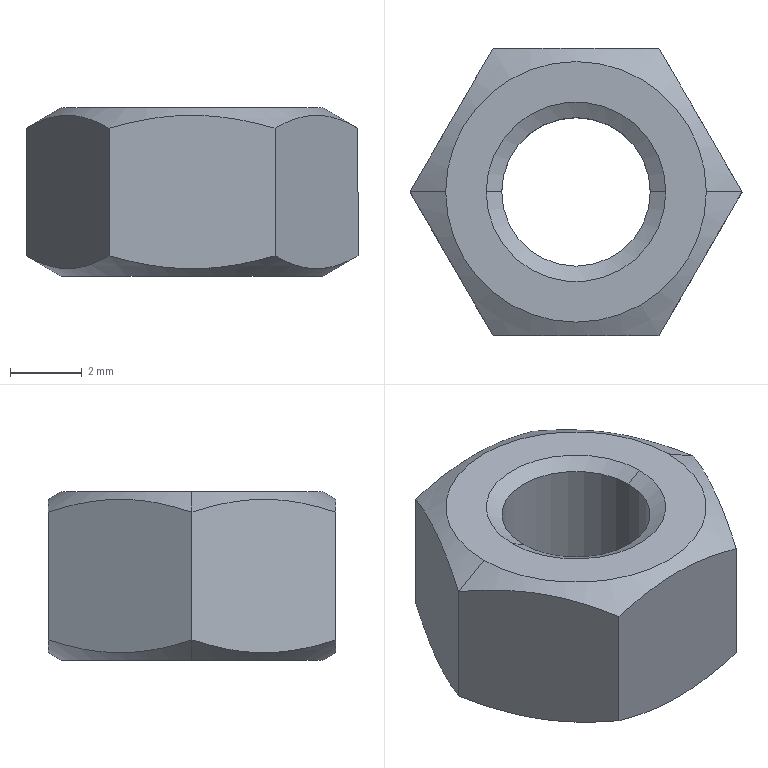Part | SolidWorks | features RevCut 2, Chamfer 1, Extrusion 1, LPattern 1 | 1 solid | 18 faces | box 9.238 x 8 x 4.7 mm | volume 190.603 mm3 | cone 8 | plane 8 | cylinder 2 | commonest cylinder face diameters 4.134 x2
STEP:
#1=CARTESIAN_POINT('',(-2.067,0.,-0.25));
#2=VERTEX_POINT('',#1);
#3=CARTESIAN_POINT('',(2.067,0.,-0.25));
#4=VERTEX_POINT('',#3);
#5=CARTESIAN_POINT('',(0.,0.,-0.25));
#6=DIRECTION('',(0.,0.,1.));
#7=DIRECTION('',(-1.,0.,0.));
#8=AXIS2_PLACEMENT_3D('',#5,#6,#7);
#9=CIRCLE('',#8,2.067);
#10=EDGE_CURVE('',#2,#4,#9,.T.);
#11=ORIENTED_EDGE('',*,*,#10,.F.);
#12=CARTESIAN_POINT('',(-2.5,0.,0.));
#13=VERTEX_POINT('',#12);
#14=CARTESIAN_POINT('',(-2.067,0.,-0.25));
#15=DIRECTION('',(-0.866,0.,0.5));
#16=VECTOR('',#15,1000.);
#17=LINE('',#14,#16);
#18=EDGE_CURVE('',#2,#13,#17,.T.);
#19=ORIENTED_EDGE('',*,*,#18,.T.);
#20=CARTESIAN_POINT('',(2.5,0.,0.));
#21=VERTEX_POINT('',#20);
#22=CARTESIAN_POINT('',(0.,0.,0.));
#23=DIRECTION('',(0.,0.,-1.));
#24=DIRECTION('',(-1.,0.,0.));
#25=AXIS2_PLACEMENT_3D('',#22,#23,#24);
#26=CIRCLE('',#25,2.5);
#27=EDGE_CURVE('',#21,#13,#26,.T.);
#28=ORIENTED_EDGE('',*,*,#27,.F.);
#29=CARTESIAN_POINT('',(2.067,0.,-0.25));
#30=DIRECTION('',(0.866,0.,0.5));
#31=VECTOR('',#30,1000.);
#32=LINE('',#29,#31);
#33=EDGE_CURVE('',#4,#21,#32,.T.);
#34=ORIENTED_EDGE('',*,*,#33,.F.);
#35=EDGE_LOOP('',(#11,#19,#28,#34));
#36=FACE_OUTER_BOUND('',#35,.T.);
#37=CARTESIAN_POINT('',(0.,0.,-0.25));
#38=DIRECTION('',(0.,0.,1.));
#39=DIRECTION('',(1.,0.,0.));
#40=AXIS2_PLACEMENT_3D('',#37,#38,#39);
#41=CONICAL_SURFACE('',#40,2.067,1.047);
#42=ADVANCED_FACE('',(#36),#41,.F.);
#43=CARTESIAN_POINT('',(2.067,0.,-4.267));
#44=VERTEX_POINT('',#43);
#45=CARTESIAN_POINT('',(-2.067,0.,-4.267));
#46=VERTEX_POINT('',#45);
#47=CARTESIAN_POINT('',(0.,0.,-4.267));
#48=DIRECTION('',(0.,0.,-1.));
#49=DIRECTION('',(-1.,0.,0.));
#50=AXIS2_PLACEMENT_3D('',#47,#48,#49);
#51=CIRCLE('',#50,2.067);
#52=EDGE_CURVE('',#44,#46,#51,.T.);
#53=ORIENTED_EDGE('',*,*,#52,.F.);
#54=CARTESIAN_POINT('',(2.317,0.,-4.7));
#55=VERTEX_POINT('',#54);
#56=CARTESIAN_POINT('',(2.317,0.,-4.7));
#57=DIRECTION('',(0.5,0.,-0.866));
#58=VECTOR('',#57,1000.);
#59=LINE('',#56,#58);
#60=EDGE_CURVE('',#44,#55,#59,.T.);
#61=ORIENTED_EDGE('',*,*,#60,.T.);
#62=CARTESIAN_POINT('',(-2.317,0.,-4.7));
#63=VERTEX_POINT('',#62);
#64=CARTESIAN_POINT('',(0.,0.,-4.7));
#65=DIRECTION('',(0.,0.,1.));
#66=DIRECTION('',(-1.,0.,0.));
#67=AXIS2_PLACEMENT_3D('',#64,#65,#66);
#68=CIRCLE('',#67,2.317);
#69=EDGE_CURVE('',#63,#55,#68,.T.);
#70=ORIENTED_EDGE('',*,*,#69,.F.);
#71=CARTESIAN_POINT('',(-2.317,0.,-4.7));
#72=DIRECTION('',(-0.5,0.,-0.866));
#73=VECTOR('',#72,1000.);
#74=LINE('',#71,#73);
#75=EDGE_CURVE('',#46,#63,#74,.T.);
#76=ORIENTED_EDGE('',*,*,#75,.F.);
#77=EDGE_LOOP('',(#53,#61,#70,#76));
#78=FACE_OUTER_BOUND('',#77,.T.);
#79=CARTESIAN_POINT('',(0.,0.,-4.7));
#80=DIRECTION('',(0.,0.,-1.));
#81=DIRECTION('',(-1.,0.,0.));
#82=AXIS2_PLACEMENT_3D('',#79,#80,#81);
#83=CONICAL_SURFACE('',#82,2.317,0.5236);
#84=ADVANCED_FACE('',(#78),#83,.F.);
#85=CARTESIAN_POINT('',(-3.625,0.,0.));
#86=VERTEX_POINT('',#85);
#87=CARTESIAN_POINT('',(3.625,0.,0.));
#88=VERTEX_POINT('',#87);
#89=CARTESIAN_POINT('',(0.,0.,0.));
#90=DIRECTION('',(0.,0.,-1.));
#91=DIRECTION('',(-1.,0.,0.));
#92=AXIS2_PLACEMENT_3D('',#89,#90,#91);
#93=CIRCLE('',#92,3.625);
#94=EDGE_CURVE('',#86,#88,#93,.T.);
#95=ORIENTED_EDGE('',*,*,#94,.T.);
#96=CARTESIAN_POINT('',(4.619,0.,-0.5738));
#97=VERTEX_POINT('',#96);
#98=CARTESIAN_POINT('',(3.625,0.,0.));
#99=DIRECTION('',(0.866,0.,-0.5));
#100=VECTOR('',#99,1000.);
#101=LINE('',#98,#100);
#102=EDGE_CURVE('',#88,#97,#101,.T.);
#103=ORIENTED_EDGE('',*,*,#102,.T.);
#104=CARTESIAN_POINT('',(2.309,4.,-0.5738));
#105=VERTEX_POINT('',#104);
#106=CARTESIAN_POINT('',(4.619,0.,-0.5738));
#107=CARTESIAN_POINT('',(4.242,0.6531,-0.3561));
#108=CARTESIAN_POINT('',(3.859,1.316,-0.217));
#109=CARTESIAN_POINT('',(3.27,2.336,-0.2163));
#110=CARTESIAN_POINT('',(3.074,2.676,-0.2504));
#111=CARTESIAN_POINT('',(2.689,3.343,-0.3748));
#112=CARTESIAN_POINT('',(2.498,3.673,-0.4648));
#113=CARTESIAN_POINT('',(2.309,4.,-0.5738));
#114=B_SPLINE_CURVE_WITH_KNOTS('',3,(#106,#107,#108,#109,#110,#111,#112,#113),.UNSPECIFIED.,.F.,.F.,(4,2,2,4),(0.000000238,0.002333,0.003499,0.004665),.UNSPECIFIED.);
#115=EDGE_CURVE('',#97,#105,#114,.T.);
#116=ORIENTED_EDGE('',*,*,#115,.T.);
#117=CARTESIAN_POINT('',(-2.309,4.,-0.5738));
#118=VERTEX_POINT('',#117);
#119=CARTESIAN_POINT('',(2.309,4.,-0.5738));
#120=CARTESIAN_POINT('',(1.936,4.,-0.466));
#121=CARTESIAN_POINT('',(1.558,4.,-0.3762));
#122=CARTESIAN_POINT('',(0.7865,4.,-0.251));
#123=CARTESIAN_POINT('',(0.3909,4.,-0.2165));
#124=CARTESIAN_POINT('',(-0.3896,4.,-0.2165));
#125=CARTESIAN_POINT('',(-0.7775,4.,-0.25));
#126=CARTESIAN_POINT('',(-1.549,4.,-0.3744));
#127=CARTESIAN_POINT('',(-1.934,4.,-0.4653));
#128=CARTESIAN_POINT('',(-2.309,4.,-0.5738));
#129=B_SPLINE_CURVE_WITH_KNOTS('',3,(#119,#120,#121,#122,#123,#124,#125,#126,#127,#128),.UNSPECIFIED.,.F.,.F.,(4,2,2,2,4),(0.001729,0.002894,0.00406,0.005225,0.006391),.UNSPECIFIED.);
#130=EDGE_CURVE('',#105,#118,#129,.T.);
#131=ORIENTED_EDGE('',*,*,#130,.T.);
#132=CARTESIAN_POINT('',(-4.619,0.,-0.5738));
#133=VERTEX_POINT('',#132);
#134=CARTESIAN_POINT('',(-2.309,4.,-0.5738));
#135=CARTESIAN_POINT('',(-2.686,3.347,-0.3561));
#136=CARTESIAN_POINT('',(-3.069,2.684,-0.217));
#137=CARTESIAN_POINT('',(-3.658,1.664,-0.2163));
#138=CARTESIAN_POINT('',(-3.854,1.324,-0.2504));
#139=CARTESIAN_POINT('',(-4.24,0.6567,-0.3748));
#140=CARTESIAN_POINT('',(-4.43,0.327,-0.4648));
#141=CARTESIAN_POINT('',(-4.619,0.,-0.5738));
#142=B_SPLINE_CURVE_WITH_KNOTS('',3,(#134,#135,#136,#137,#138,#139,#140,#141),.UNSPECIFIED.,.F.,.F.,(4,2,2,4),(0.000000238,0.002333,0.003499,0.004665),.UNSPECIFIED.);
#143=EDGE_CURVE('',#118,#133,#142,.T.);
#144=ORIENTED_EDGE('',*,*,#143,.T.);
#145=CARTESIAN_POINT('',(-3.625,0.,0.));
#146=DIRECTION('',(-0.866,0.,-0.5));
#147=VECTOR('',#146,1000.);
#148=LINE('',#145,#147);
#149=EDGE_CURVE('',#86,#133,#148,.T.);
#150=ORIENTED_EDGE('',*,*,#149,.F.);
#151=EDGE_LOOP('',(#95,#103,#116,#131,#144,#150));
#152=FACE_OUTER_BOUND('',#151,.T.);
#153=CARTESIAN_POINT('',(0.,0.,0.));
#154=DIRECTION('',(0.,0.,-1.));
#155=DIRECTION('',(-1.,0.,0.));
#156=AXIS2_PLACEMENT_3D('',#153,#154,#155);
#157=CONICAL_SURFACE('',#156,3.625,1.047);
#158=ADVANCED_FACE('',(#152),#157,.T.);
#159=CARTESIAN_POINT('',(-3.625,0.,-4.7));
#160=VERTEX_POINT('',#159);
#161=CARTESIAN_POINT('',(3.625,0.,-4.7));
#162=VERTEX_POINT('',#161);
#163=CARTESIAN_POINT('',(0.,0.,-4.7));
#164=DIRECTION('',(0.,0.,-1.));
#165=DIRECTION('',(-1.,0.,0.));
#166=AXIS2_PLACEMENT_3D('',#163,#164,#165);
#167=CIRCLE('',#166,3.625);
#168=EDGE_CURVE('',#160,#162,#167,.T.);
#169=ORIENTED_EDGE('',*,*,#168,.F.);
#170=CARTESIAN_POINT('',(-4.619,0.,-4.126));
#171=VERTEX_POINT('',#170);
#172=CARTESIAN_POINT('',(-4.619,0.,-4.126));
#173=DIRECTION('',(-0.866,0.,0.5));
#174=VECTOR('',#173,1000.);
#175=LINE('',#172,#174);
#176=EDGE_CURVE('',#160,#171,#175,.T.);
#177=ORIENTED_EDGE('',*,*,#176,.T.);
#178=CARTESIAN_POINT('',(-2.309,4.,-4.126));
#179=VERTEX_POINT('',#178);
#180=CARTESIAN_POINT('',(-4.619,0.,-4.126));
#181=CARTESIAN_POINT('',(-4.242,0.6531,-4.344));
#182=CARTESIAN_POINT('',(-3.859,1.316,-4.483));
#183=CARTESIAN_POINT('',(-3.27,2.336,-4.484));
#184=CARTESIAN_POINT('',(-3.074,2.676,-4.45));
#185=CARTESIAN_POINT('',(-2.689,3.343,-4.325));
#186=CARTESIAN_POINT('',(-2.498,3.673,-4.235));
#187=CARTESIAN_POINT('',(-2.309,4.,-4.126));
#188=B_SPLINE_CURVE_WITH_KNOTS('',3,(#180,#181,#182,#183,#184,#185,#186,#187),.UNSPECIFIED.,.F.,.F.,(4,2,2,4),(0.000000238,0.002333,0.003499,0.004665),.UNSPECIFIED.);
#189=EDGE_CURVE('',#171,#179,#188,.T.);
#190=ORIENTED_EDGE('',*,*,#189,.T.);
#191=CARTESIAN_POINT('',(2.309,4.,-4.126));
#192=VERTEX_POINT('',#191);
#193=CARTESIAN_POINT('',(-2.309,4.,-4.126));
#194=CARTESIAN_POINT('',(-1.934,4.,-4.235));
#195=CARTESIAN_POINT('',(-1.549,4.,-4.326));
#196=CARTESIAN_POINT('',(-0.7775,4.,-4.45));
#197=CARTESIAN_POINT('',(-0.3896,4.,-4.484));
#198=CARTESIAN_POINT('',(0.3909,4.,-4.483));
#199=CARTESIAN_POINT('',(0.7865,4.,-4.449));
#200=CARTESIAN_POINT('',(1.558,4.,-4.324));
#201=CARTESIAN_POINT('',(1.936,4.,-4.234));
#202=CARTESIAN_POINT('',(2.309,4.,-4.126));
#203=B_SPLINE_CURVE_WITH_KNOTS('',3,(#193,#194,#195,#196,#197,#198,#199,#200,#201,#202),.UNSPECIFIED.,.F.,.F.,(4,2,2,2,4),(0.004087,0.005255,0.006424,0.007592,0.00876),.UNSPECIFIED.);
#204=EDGE_CURVE('',#179,#192,#203,.T.);
#205=ORIENTED_EDGE('',*,*,#204,.T.);
#206=CARTESIAN_POINT('',(4.619,0.,-4.126));
#207=VERTEX_POINT('',#206);
#208=CARTESIAN_POINT('',(2.309,4.,-4.126));
#209=CARTESIAN_POINT('',(2.686,3.347,-4.344));
#210=CARTESIAN_POINT('',(3.069,2.684,-4.483));
#211=CARTESIAN_POINT('',(3.658,1.664,-4.484));
#212=CARTESIAN_POINT('',(3.854,1.324,-4.45));
#213=CARTESIAN_POINT('',(4.24,0.6567,-4.325));
#214=CARTESIAN_POINT('',(4.43,0.327,-4.235));
#215=CARTESIAN_POINT('',(4.619,0.,-4.126));
#216=B_SPLINE_CURVE_WITH_KNOTS('',3,(#208,#209,#210,#211,#212,#213,#214,#215),.UNSPECIFIED.,.F.,.F.,(4,2,2,4),(0.000000238,0.002333,0.003499,0.004665),.UNSPECIFIED.);
#217=EDGE_CURVE('',#192,#207,#216,.T.);
#218=ORIENTED_EDGE('',*,*,#217,.T.);
#219=CARTESIAN_POINT('',(4.619,0.,-4.126));
#220=DIRECTION('',(0.866,0.,0.5));
#221=VECTOR('',#220,1000.);
#222=LINE('',#219,#221);
#223=EDGE_CURVE('',#162,#207,#222,.T.);
#224=ORIENTED_EDGE('',*,*,#223,.F.);
#225=EDGE_LOOP('',(#169,#177,#190,#205,#218,#224));
#226=FACE_OUTER_BOUND('',#225,.T.);
#227=CARTESIAN_POINT('',(0.,0.,-4.126));
#228=DIRECTION('',(0.,0.,1.));
#229=DIRECTION('',(1.,0.,0.));
#230=AXIS2_PLACEMENT_3D('',#227,#228,#229);
#231=CONICAL_SURFACE('',#230,4.619,1.047);
#232=ADVANCED_FACE('',(#226),#231,.T.);
#233=ORIENTED_EDGE('',*,*,#52,.T.);
#234=CARTESIAN_POINT('',(-2.067,0.,-4.7));
#235=DIRECTION('',(0.,0.,1.));
#236=VECTOR('',#235,1000.);
#237=LINE('',#234,#236);
#238=EDGE_CURVE('',#46,#2,#237,.T.);
#239=ORIENTED_EDGE('',*,*,#238,.T.);
#240=ORIENTED_EDGE('',*,*,#10,.T.);
#241=CARTESIAN_POINT('',(2.067,0.,-4.7));
#242=DIRECTION('',(0.,0.,1.));
#243=VECTOR('',#242,1000.);
#244=LINE('',#241,#243);
#245=EDGE_CURVE('',#44,#4,#244,.T.);
#246=ORIENTED_EDGE('',*,*,#245,.F.);
#247=EDGE_LOOP('',(#233,#239,#240,#246));
#248=FACE_OUTER_BOUND('',#247,.T.);
#249=CARTESIAN_POINT('',(0.,0.,-4.7));
#250=DIRECTION('',(0.,0.,1.));
#251=DIRECTION('',(1.,0.,0.));
#252=AXIS2_PLACEMENT_3D('',#249,#250,#251);
#253=CYLINDRICAL_SURFACE('',#252,2.067);
#254=ADVANCED_FACE('',(#248),#253,.F.);
#255=CARTESIAN_POINT('',(2.309,-4.,-0.5738));
#256=VERTEX_POINT('',#255);
#257=CARTESIAN_POINT('',(2.309,-4.,-0.5738));
#258=CARTESIAN_POINT('',(2.686,-3.347,-0.3561));
#259=CARTESIAN_POINT('',(3.069,-2.684,-0.217));
#260=CARTESIAN_POINT('',(3.658,-1.664,-0.2163));
#261=CARTESIAN_POINT('',(3.854,-1.324,-0.2504));
#262=CARTESIAN_POINT('',(4.24,-0.6567,-0.3748));
#263=CARTESIAN_POINT('',(4.43,-0.327,-0.4648));
#264=CARTESIAN_POINT('',(4.619,0.,-0.5738));
#265=B_SPLINE_CURVE_WITH_KNOTS('',3,(#257,#258,#259,#260,#261,#262,#263,#264),.UNSPECIFIED.,.F.,.F.,(4,2,2,4),(0.000000238,0.002333,0.003499,0.004665),.UNSPECIFIED.);
#266=EDGE_CURVE('',#256,#97,#265,.T.);
#267=ORIENTED_EDGE('',*,*,#266,.F.);
#268=CARTESIAN_POINT('',(2.309,-4.,-4.126));
#269=VERTEX_POINT('',#268);
#270=CARTESIAN_POINT('',(2.309,-4.,-4.7));
#271=DIRECTION('',(0.,0.,1.));
#272=VECTOR('',#271,1000.);
#273=LINE('',#270,#272);
#274=EDGE_CURVE('',#269,#256,#273,.T.);
#275=ORIENTED_EDGE('',*,*,#274,.F.);
#276=CARTESIAN_POINT('',(4.619,0.,-4.126));
#277=CARTESIAN_POINT('',(4.242,-0.6531,-4.344));
#278=CARTESIAN_POINT('',(3.859,-1.316,-4.483));
#279=CARTESIAN_POINT('',(3.27,-2.336,-4.484));
#280=CARTESIAN_POINT('',(3.074,-2.676,-4.45));
#281=CARTESIAN_POINT('',(2.689,-3.343,-4.325));
#282=CARTESIAN_POINT('',(2.498,-3.673,-4.235));
#283=CARTESIAN_POINT('',(2.309,-4.,-4.126));
#284=B_SPLINE_CURVE_WITH_KNOTS('',3,(#276,#277,#278,#279,#280,#281,#282,#283),.UNSPECIFIED.,.F.,.F.,(4,2,2,4),(0.000000238,0.002333,0.003499,0.004665),.UNSPECIFIED.);
#285=EDGE_CURVE('',#207,#269,#284,.T.);
#286=ORIENTED_EDGE('',*,*,#285,.F.);
#287=CARTESIAN_POINT('',(4.619,0.,-4.7));
#288=DIRECTION('',(0.,0.,1.));
#289=VECTOR('',#288,1000.);
#290=LINE('',#287,#289);
#291=EDGE_CURVE('',#207,#97,#290,.T.);
#292=ORIENTED_EDGE('',*,*,#291,.T.);
#293=EDGE_LOOP('',(#267,#275,#286,#292));
#294=FACE_OUTER_BOUND('',#293,.T.);
#295=CARTESIAN_POINT('',(2.309,-4.,-4.7));
#296=DIRECTION('',(0.866,-0.5,0.));
#297=DIRECTION('',(0.5,0.866,0.));
#298=AXIS2_PLACEMENT_3D('',#295,#296,#297);
#299=PLANE('',#298);
#300=ADVANCED_FACE('',(#294),#299,.T.);
#301=CARTESIAN_POINT('',(-2.309,-4.,-0.5738));
#302=VERTEX_POINT('',#301);
#303=CARTESIAN_POINT('',(-2.309,-4.,-0.5738));
#304=CARTESIAN_POINT('',(-1.934,-4.,-0.4653));
#305=CARTESIAN_POINT('',(-1.549,-4.,-0.3744));
#306=CARTESIAN_POINT('',(-0.7775,-4.,-0.25));
#307=CARTESIAN_POINT('',(-0.3896,-4.,-0.2165));
#308=CARTESIAN_POINT('',(0.3909,-4.,-0.2165));
#309=CARTESIAN_POINT('',(0.7865,-4.,-0.251));
#310=CARTESIAN_POINT('',(1.558,-4.,-0.3762));
#311=CARTESIAN_POINT('',(1.936,-4.,-0.466));
#312=CARTESIAN_POINT('',(2.309,-4.,-0.5738));
#313=B_SPLINE_CURVE_WITH_KNOTS('',3,(#303,#304,#305,#306,#307,#308,#309,#310,#311,#312),.UNSPECIFIED.,.F.,.F.,(4,2,2,2,4),(0.004087,0.005255,0.006424,0.007592,0.00876),.UNSPECIFIED.);
#314=EDGE_CURVE('',#302,#256,#313,.T.);
#315=ORIENTED_EDGE('',*,*,#314,.F.);
#316=CARTESIAN_POINT('',(-2.309,-4.,-4.126));
#317=VERTEX_POINT('',#316);
#318=CARTESIAN_POINT('',(-2.309,-4.,-4.7));
#319=DIRECTION('',(0.,0.,1.));
#320=VECTOR('',#319,1000.);
#321=LINE('',#318,#320);
#322=EDGE_CURVE('',#317,#302,#321,.T.);
#323=ORIENTED_EDGE('',*,*,#322,.F.);
#324=CARTESIAN_POINT('',(2.309,-4.,-4.126));
#325=CARTESIAN_POINT('',(1.936,-4.,-4.234));
#326=CARTESIAN_POINT('',(1.558,-4.,-4.324));
#327=CARTESIAN_POINT('',(0.7865,-4.,-4.449));
#328=CARTESIAN_POINT('',(0.3909,-4.,-4.483));
#329=CARTESIAN_POINT('',(-0.3896,-4.,-4.484));
#330=CARTESIAN_POINT('',(-0.7775,-4.,-4.45));
#331=CARTESIAN_POINT('',(-1.549,-4.,-4.326));
#332=CARTESIAN_POINT('',(-1.934,-4.,-4.235));
#333=CARTESIAN_POINT('',(-2.309,-4.,-4.126));
#334=B_SPLINE_CURVE_WITH_KNOTS('',3,(#324,#325,#326,#327,#328,#329,#330,#331,#332,#333),.UNSPECIFIED.,.F.,.F.,(4,2,2,2,4),(0.001729,0.002894,0.00406,0.005225,0.006391),.UNSPECIFIED.);
#335=EDGE_CURVE('',#269,#317,#334,.T.);
#336=ORIENTED_EDGE('',*,*,#335,.F.);
#337=ORIENTED_EDGE('',*,*,#274,.T.);
#338=EDGE_LOOP('',(#315,#323,#336,#337));
#339=FACE_OUTER_BOUND('',#338,.T.);
#340=CARTESIAN_POINT('',(-2.309,-4.,-4.7));
#341=DIRECTION('',(0.,-1.,0.));
#342=DIRECTION('',(0.,0.,-1.));
#343=AXIS2_PLACEMENT_3D('',#340,#341,#342);
#344=PLANE('',#343);
#345=ADVANCED_FACE('',(#339),#344,.T.);
#346=CARTESIAN_POINT('',(-4.619,0.,-0.5738));
#347=CARTESIAN_POINT('',(-4.242,-0.6531,-0.3561));
#348=CARTESIAN_POINT('',(-3.859,-1.316,-0.217));
#349=CARTESIAN_POINT('',(-3.27,-2.336,-0.2163));
#350=CARTESIAN_POINT('',(-3.074,-2.676,-0.2504));
#351=CARTESIAN_POINT('',(-2.689,-3.343,-0.3748));
#352=CARTESIAN_POINT('',(-2.498,-3.673,-0.4648));
#353=CARTESIAN_POINT('',(-2.309,-4.,-0.5738));
#354=B_SPLINE_CURVE_WITH_KNOTS('',3,(#346,#347,#348,#349,#350,#351,#352,#353),.UNSPECIFIED.,.F.,.F.,(4,2,2,4),(0.000000238,0.002333,0.003499,0.004665),.UNSPECIFIED.);
#355=EDGE_CURVE('',#133,#302,#354,.T.);
#356=ORIENTED_EDGE('',*,*,#355,.F.);
#357=CARTESIAN_POINT('',(-4.619,0.,-4.7));
#358=DIRECTION('',(0.,0.,1.));
#359=VECTOR('',#358,1000.);
#360=LINE('',#357,#359);
#361=EDGE_CURVE('',#171,#133,#360,.T.);
#362=ORIENTED_EDGE('',*,*,#361,.F.);
#363=CARTESIAN_POINT('',(-2.309,-4.,-4.126));
#364=CARTESIAN_POINT('',(-2.686,-3.347,-4.344));
#365=CARTESIAN_POINT('',(-3.069,-2.684,-4.483));
#366=CARTESIAN_POINT('',(-3.658,-1.664,-4.484));
#367=CARTESIAN_POINT('',(-3.854,-1.324,-4.45));
#368=CARTESIAN_POINT('',(-4.24,-0.6567,-4.325));
#369=CARTESIAN_POINT('',(-4.43,-0.327,-4.235));
#370=CARTESIAN_POINT('',(-4.619,0.,-4.126));
#371=B_SPLINE_CURVE_WITH_KNOTS('',3,(#363,#364,#365,#366,#367,#368,#369,#370),.UNSPECIFIED.,.F.,.F.,(4,2,2,4),(0.000000238,0.002333,0.003499,0.004665),.UNSPECIFIED.);
#372=EDGE_CURVE('',#317,#171,#371,.T.);
#373=ORIENTED_EDGE('',*,*,#372,.F.);
#374=ORIENTED_EDGE('',*,*,#322,.T.);
#375=EDGE_LOOP('',(#356,#362,#373,#374));
#376=FACE_OUTER_BOUND('',#375,.T.);
#377=CARTESIAN_POINT('',(-4.619,0.,-4.7));
#378=DIRECTION('',(-0.866,-0.5,0.));
#379=DIRECTION('',(0.5,-0.866,0.));
#380=AXIS2_PLACEMENT_3D('',#377,#378,#379);
#381=PLANE('',#380);
#382=ADVANCED_FACE('',(#376),#381,.T.);
#383=ORIENTED_EDGE('',*,*,#143,.F.);
#384=CARTESIAN_POINT('',(-2.309,4.,-4.7));
#385=DIRECTION('',(0.,0.,1.));
#386=VECTOR('',#385,1000.);
#387=LINE('',#384,#386);
#388=EDGE_CURVE('',#179,#118,#387,.T.);
#389=ORIENTED_EDGE('',*,*,#388,.F.);
#390=ORIENTED_EDGE('',*,*,#189,.F.);
#391=ORIENTED_EDGE('',*,*,#361,.T.);
#392=EDGE_LOOP('',(#383,#389,#390,#391));
#393=FACE_OUTER_BOUND('',#392,.T.);
#394=CARTESIAN_POINT('',(-2.309,4.,-4.7));
#395=DIRECTION('',(-0.866,0.5,0.));
#396=DIRECTION('',(-0.5,-0.866,0.));
#397=AXIS2_PLACEMENT_3D('',#394,#395,#396);
#398=PLANE('',#397);
#399=ADVANCED_FACE('',(#393),#398,.T.);
#400=ORIENTED_EDGE('',*,*,#130,.F.);
#401=CARTESIAN_POINT('',(2.309,4.,-4.7));
#402=DIRECTION('',(0.,0.,1.));
#403=VECTOR('',#402,1000.);
#404=LINE('',#401,#403);
#405=EDGE_CURVE('',#192,#105,#404,.T.);
#406=ORIENTED_EDGE('',*,*,#405,.F.);
#407=ORIENTED_EDGE('',*,*,#204,.F.);
#408=ORIENTED_EDGE('',*,*,#388,.T.);
#409=EDGE_LOOP('',(#400,#406,#407,#408));
#410=FACE_OUTER_BOUND('',#409,.T.);
#411=CARTESIAN_POINT('',(2.309,4.,-4.7));
#412=DIRECTION('',(0.,1.,0.));
#413=DIRECTION('',(-1.,0.,0.));
#414=AXIS2_PLACEMENT_3D('',#411,#412,#413);
#415=PLANE('',#414);
#416=ADVANCED_FACE('',(#410),#415,.T.);
#417=ORIENTED_EDGE('',*,*,#115,.F.);
#418=ORIENTED_EDGE('',*,*,#291,.F.);
#419=ORIENTED_EDGE('',*,*,#217,.F.);
#420=ORIENTED_EDGE('',*,*,#405,.T.);
#421=EDGE_LOOP('',(#417,#418,#419,#420));
#422=FACE_OUTER_BOUND('',#421,.T.);
#423=CARTESIAN_POINT('',(4.619,0.,-4.7));
#424=DIRECTION('',(0.866,0.5,0.));
#425=DIRECTION('',(-0.5,0.866,0.));
#426=AXIS2_PLACEMENT_3D('',#423,#424,#425);
#427=PLANE('',#426);
#428=ADVANCED_FACE('',(#422),#427,.T.);
#429=ORIENTED_EDGE('',*,*,#69,.T.);
#430=CARTESIAN_POINT('',(0.,0.,-4.7));
#431=DIRECTION('',(0.,0.,1.));
#432=DIRECTION('',(-1.,0.,0.));
#433=AXIS2_PLACEMENT_3D('',#430,#431,#432);
#434=CIRCLE('',#433,2.317);
#435=EDGE_CURVE('',#55,#63,#434,.T.);
#436=ORIENTED_EDGE('',*,*,#435,.T.);
#437=EDGE_LOOP('',(#429,#436));
#438=FACE_BOUND('',#437,.T.);
#439=CARTESIAN_POINT('',(0.,0.,-4.7));
#440=DIRECTION('',(0.,0.,-1.));
#441=DIRECTION('',(-1.,0.,0.));
#442=AXIS2_PLACEMENT_3D('',#439,#440,#441);
#443=CIRCLE('',#442,3.625);
#444=EDGE_CURVE('',#162,#160,#443,.T.);
#445=ORIENTED_EDGE('',*,*,#444,.T.);
#446=ORIENTED_EDGE('',*,*,#168,.T.);
#447=EDGE_LOOP('',(#445,#446));
#448=FACE_OUTER_BOUND('',#447,.T.);
#449=CARTESIAN_POINT('',(0.,-8.,-4.7));
#450=DIRECTION('',(0.,0.,-1.));
#451=DIRECTION('',(-1.,0.,0.));
#452=AXIS2_PLACEMENT_3D('',#449,#450,#451);
#453=PLANE('',#452);
#454=ADVANCED_FACE('',(#438,#448),#453,.T.);
#455=ORIENTED_EDGE('',*,*,#27,.T.);
#456=CARTESIAN_POINT('',(0.,0.,0.));
#457=DIRECTION('',(0.,0.,-1.));
#458=DIRECTION('',(-1.,0.,0.));
#459=AXIS2_PLACEMENT_3D('',#456,#457,#458);
#460=CIRCLE('',#459,2.5);
#461=EDGE_CURVE('',#13,#21,#460,.T.);
#462=ORIENTED_EDGE('',*,*,#461,.T.);
#463=EDGE_LOOP('',(#455,#462));
#464=FACE_BOUND('',#463,.T.);
#465=ORIENTED_EDGE('',*,*,#94,.F.);
#466=CARTESIAN_POINT('',(0.,0.,0.));
#467=DIRECTION('',(0.,0.,-1.));
#468=DIRECTION('',(-1.,0.,0.));
#469=AXIS2_PLACEMENT_3D('',#466,#467,#468);
#470=CIRCLE('',#469,3.625);
#471=EDGE_CURVE('',#88,#86,#470,.T.);
#472=ORIENTED_EDGE('',*,*,#471,.F.);
#473=EDGE_LOOP('',(#465,#472));
#474=FACE_OUTER_BOUND('',#473,.T.);
#475=CARTESIAN_POINT('',(0.,-8.,0.));
#476=DIRECTION('',(0.,0.,-1.));
#477=DIRECTION('',(-1.,0.,0.));
#478=AXIS2_PLACEMENT_3D('',#475,#476,#477);
#479=PLANE('',#478);
#480=ADVANCED_FACE('',(#464,#474),#479,.F.);
#481=ORIENTED_EDGE('',*,*,#238,.F.);
#482=CARTESIAN_POINT('',(0.,0.,-4.267));
#483=DIRECTION('',(0.,0.,-1.));
#484=DIRECTION('',(-1.,0.,0.));
#485=AXIS2_PLACEMENT_3D('',#482,#483,#484);
#486=CIRCLE('',#485,2.067);
#487=EDGE_CURVE('',#46,#44,#486,.T.);
#488=ORIENTED_EDGE('',*,*,#487,.T.);
#489=ORIENTED_EDGE('',*,*,#245,.T.);
#490=CARTESIAN_POINT('',(0.,0.,-0.25));
#491=DIRECTION('',(0.,0.,1.));
#492=DIRECTION('',(-1.,0.,0.));
#493=AXIS2_PLACEMENT_3D('',#490,#491,#492);
#494=CIRCLE('',#493,2.067);
#495=EDGE_CURVE('',#4,#2,#494,.T.);
#496=ORIENTED_EDGE('',*,*,#495,.T.);
#497=EDGE_LOOP('',(#481,#488,#489,#496));
#498=FACE_OUTER_BOUND('',#497,.T.);
#499=CARTESIAN_POINT('',(0.,0.,-4.7));
#500=DIRECTION('',(0.,0.,1.));
#501=DIRECTION('',(1.,0.,0.));
#502=AXIS2_PLACEMENT_3D('',#499,#500,#501);
#503=CYLINDRICAL_SURFACE('',#502,2.067);
#504=ADVANCED_FACE('',(#498),#503,.F.);
#505=ORIENTED_EDGE('',*,*,#176,.F.);
#506=ORIENTED_EDGE('',*,*,#444,.F.);
#507=ORIENTED_EDGE('',*,*,#223,.T.);
#508=ORIENTED_EDGE('',*,*,#285,.T.);
#509=ORIENTED_EDGE('',*,*,#335,.T.);
#510=ORIENTED_EDGE('',*,*,#372,.T.);
#511=EDGE_LOOP('',(#505,#506,#507,#508,#509,#510));
#512=FACE_OUTER_BOUND('',#511,.T.);
#513=CARTESIAN_POINT('',(0.,0.,-4.126));
#514=DIRECTION('',(0.,0.,1.));
#515=DIRECTION('',(1.,0.,0.));
#516=AXIS2_PLACEMENT_3D('',#513,#514,#515);
#517=CONICAL_SURFACE('',#516,4.619,1.047);
#518=ADVANCED_FACE('',(#512),#517,.T.);
#519=ORIENTED_EDGE('',*,*,#102,.F.);
#520=ORIENTED_EDGE('',*,*,#471,.T.);
#521=ORIENTED_EDGE('',*,*,#149,.T.);
#522=ORIENTED_EDGE('',*,*,#355,.T.);
#523=ORIENTED_EDGE('',*,*,#314,.T.);
#524=ORIENTED_EDGE('',*,*,#266,.T.);
#525=EDGE_LOOP('',(#519,#520,#521,#522,#523,#524));
#526=FACE_OUTER_BOUND('',#525,.T.);
#527=CARTESIAN_POINT('',(0.,0.,0.));
#528=DIRECTION('',(0.,0.,-1.));
#529=DIRECTION('',(-1.,0.,0.));
#530=AXIS2_PLACEMENT_3D('',#527,#528,#529);
#531=CONICAL_SURFACE('',#530,3.625,1.047);
#532=ADVANCED_FACE('',(#526),#531,.T.);
#533=ORIENTED_EDGE('',*,*,#60,.F.);
#534=ORIENTED_EDGE('',*,*,#487,.F.);
#535=ORIENTED_EDGE('',*,*,#75,.T.);
#536=ORIENTED_EDGE('',*,*,#435,.F.);
#537=EDGE_LOOP('',(#533,#534,#535,#536));
#538=FACE_OUTER_BOUND('',#537,.T.);
#539=CARTESIAN_POINT('',(0.,0.,-4.7));
#540=DIRECTION('',(0.,0.,-1.));
#541=DIRECTION('',(-1.,0.,0.));
#542=AXIS2_PLACEMENT_3D('',#539,#540,#541);
#543=CONICAL_SURFACE('',#542,2.317,0.5236);
#544=ADVANCED_FACE('',(#538),#543,.F.);
#545=ORIENTED_EDGE('',*,*,#18,.F.);
#546=ORIENTED_EDGE('',*,*,#495,.F.);
#547=ORIENTED_EDGE('',*,*,#33,.T.);
#548=ORIENTED_EDGE('',*,*,#461,.F.);
#549=EDGE_LOOP('',(#545,#546,#547,#548));
#550=FACE_OUTER_BOUND('',#549,.T.);
#551=CARTESIAN_POINT('',(0.,0.,-0.25));
#552=DIRECTION('',(0.,0.,1.));
#553=DIRECTION('',(1.,0.,0.));
#554=AXIS2_PLACEMENT_3D('',#551,#552,#553);
#555=CONICAL_SURFACE('',#554,2.067,1.047);
#556=ADVANCED_FACE('',(#550),#555,.F.);
#557=CLOSED_SHELL('',(#42,#84,#158,#232,#254,#300,#345,#382,#399,#416,#428,#454,#480,#504,#518,#532,#544,#556));
#558=MANIFOLD_SOLID_BREP('',#557);
#559=CARTESIAN_POINT('',(0.,0.,0.));
#560=DIRECTION('',(0.,0.,1.));
#561=DIRECTION('',(1.,0.,0.));
#562=AXIS2_PLACEMENT_3D('',#559,#560,#561);
#563=(LENGTH_UNIT()NAMED_UNIT(*)SI_UNIT(.MILLI.,.METRE.));
#564=UNCERTAINTY_MEASURE_WITH_UNIT(LENGTH_MEASURE(0.00001),#563,'','');
#565=(NAMED_UNIT(*)PLANE_ANGLE_UNIT()SI_UNIT($,.RADIAN.));
#566=(NAMED_UNIT(*)SI_UNIT($,.STERADIAN.)SOLID_ANGLE_UNIT());
#567=(GEOMETRIC_REPRESENTATION_CONTEXT(3)GLOBAL_UNCERTAINTY_ASSIGNED_CONTEXT((#564))GLOBAL_UNIT_ASSIGNED_CONTEXT((#563,#565,#566))REPRESENTATION_CONTEXT('',''));
#568=ADVANCED_BREP_SHAPE_REPRESENTATION('',(#558,#562),#567);